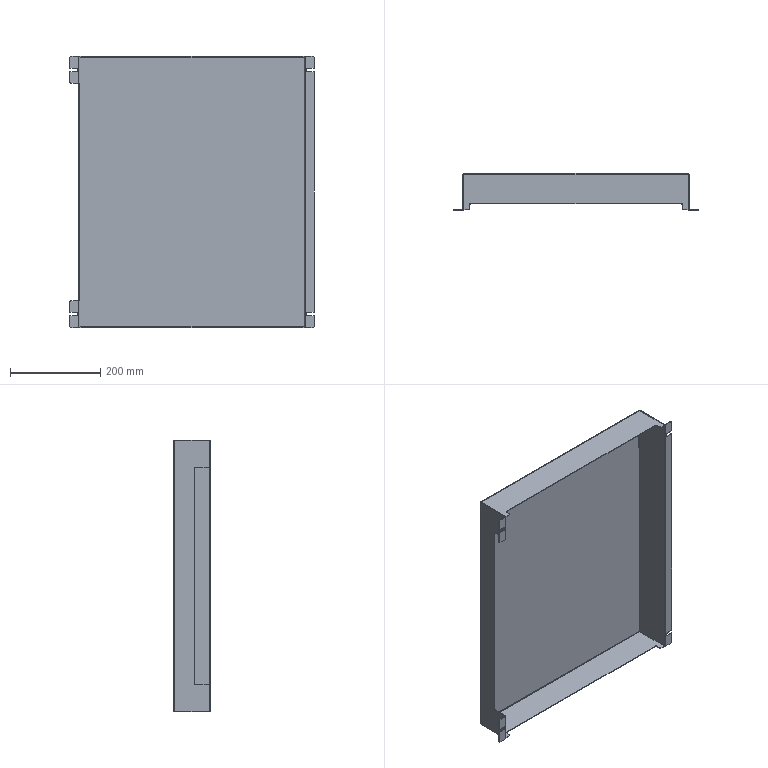Part | STEP file | cover plate43r | 1 solid | 112 faces | box 540 x 81.5 x 600 mm | volume 684567 mm3 | plane 76 | cylinder 36 | commonest cylinder face diameters 4 x16 1.473 x7 4.473 x7 7 x6